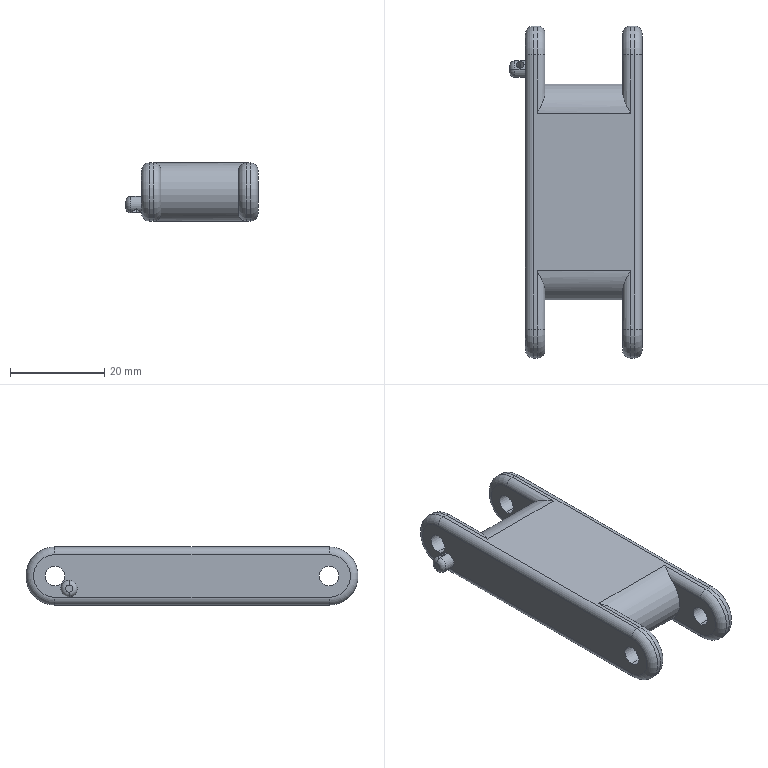Part | SolidWorks | features ICE 4, 3DProfileFeature 2, Fillet 2, Extrusion 1, Scale 1 | 1 solid | 49 faces | box 28.067 x 70.63 x 12.383 mm | volume 15312 mm3 | cylinder 30 | torus 10 | plane 9 | commonest cylinder face diameters 3.302 x12 12.383 x6 4.127 x4 4.128 x4 1.655 x2 3.516 x2